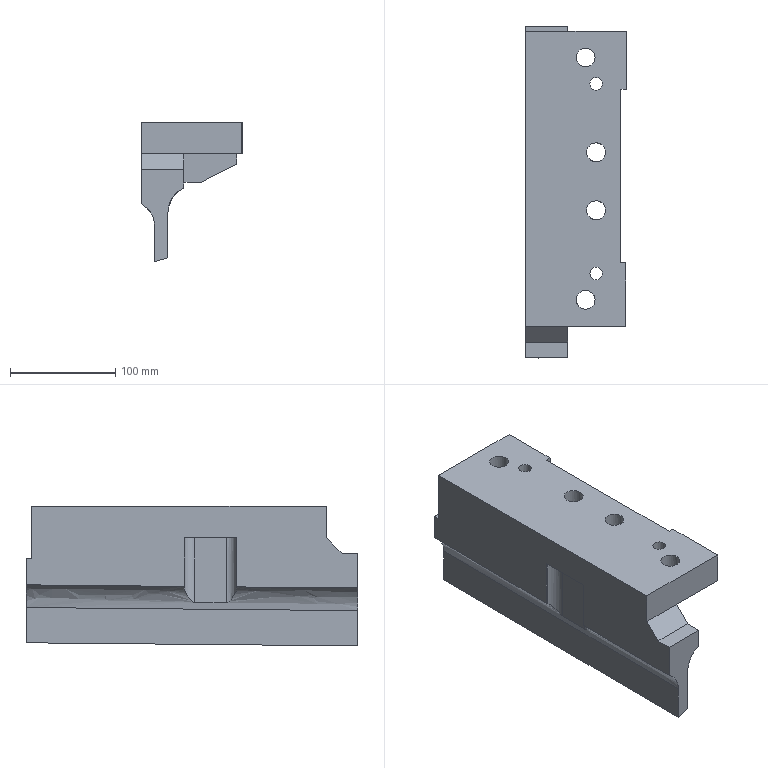Part | NX | features solid 2 | 1 solid | 57 faces | box 95.292 x 315 x 132.688 mm | volume 1485645 mm3 | plane 37 | cylinder 13 | spline 7 | commonest cylinder face diameters 18 x4 26 x4 12 x2 20 x2 10 x1